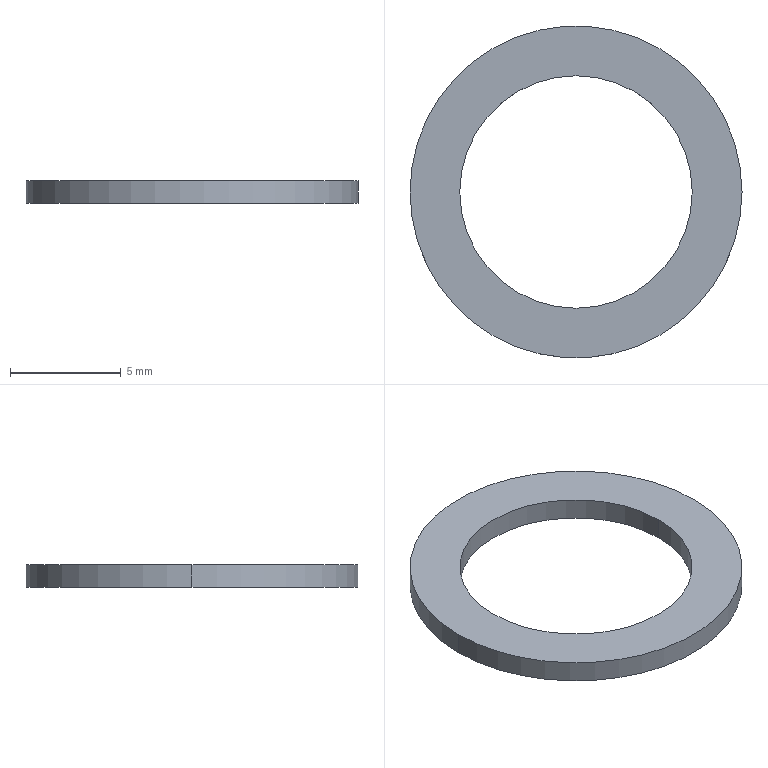Part | STEP file | BCC3 H11_5 | 1 solid | 6 faces | box 15 x 15 x 1 mm | volume 90.124 mm3 | cylinder 4 | plane 2 | commonest cylinder face diameters 10.5 x2 15 x2
STEP:
#1=CARTESIAN_POINT('',(0.,0.,0.));
#2=DIRECTION('',(0.,0.,1.));
#3=DIRECTION('',(1.,0.,0.));
#4=AXIS2_PLACEMENT_3D('',#1,#2,#3);
#5=CARTESIAN_POINT('',(-5.25,0.,1.));
#6=VERTEX_POINT('',#5);
#7=CARTESIAN_POINT('',(-5.25,0.,0.));
#8=VERTEX_POINT('',#7);
#9=CARTESIAN_POINT('',(-5.25,0.,1.));
#10=DIRECTION('',(0.,0.,-1.));
#11=VECTOR('',#10,1.);
#12=LINE('',#9,#11);
#13=CARTESIAN_POINT('',(0.,0.,1.));
#14=DIRECTION('',(0.,0.,-1.));
#15=DIRECTION('',(-1.,0.,0.));
#16=AXIS2_PLACEMENT_3D('',#13,#14,#15);
#17=CYLINDRICAL_SURFACE('',#16,5.25);
#18=CARTESIAN_POINT('',(6.283,0.));
#19=DIRECTION('',(0.,1.));
#20=VECTOR('',#19,1.);
#21=LINE('',#18,#20);
#22=(GEOMETRIC_REPRESENTATION_CONTEXT(2)PARAMETRIC_REPRESENTATION_CONTEXT()REPRESENTATION_CONTEXT('',''));
#23=DEFINITIONAL_REPRESENTATION('',(#21),#22);
#24=PCURVE('',#17,#23);
#25=CARTESIAN_POINT('',(0.,0.,1.));
#26=DIRECTION('',(0.,0.,-1.));
#27=DIRECTION('',(-1.,0.,0.));
#28=AXIS2_PLACEMENT_3D('',#25,#26,#27);
#29=CYLINDRICAL_SURFACE('',#28,5.25);
#30=CARTESIAN_POINT('',(0.,0.));
#31=DIRECTION('',(0.,1.));
#32=VECTOR('',#31,1.);
#33=LINE('',#30,#32);
#34=(GEOMETRIC_REPRESENTATION_CONTEXT(2)PARAMETRIC_REPRESENTATION_CONTEXT()REPRESENTATION_CONTEXT('',''));
#35=DEFINITIONAL_REPRESENTATION('',(#33),#34);
#36=PCURVE('',#29,#35);
#37=SURFACE_CURVE('',#12,(#24,#36),.PCURVE_S1.);
#38=EDGE_CURVE('',#6,#8,#37,.T.);
#39=ORIENTED_EDGE('',*,*,#38,.T.);
#40=CARTESIAN_POINT('',(5.25,0.,0.));
#41=VERTEX_POINT('',#40);
#42=CARTESIAN_POINT('',(0.,0.,0.));
#43=DIRECTION('',(0.,0.,1.));
#44=DIRECTION('',(1.,0.,0.));
#45=AXIS2_PLACEMENT_3D('',#42,#43,#44);
#46=CIRCLE('',#45,5.25);
#47=CARTESIAN_POINT('',(9.425,1.));
#48=DIRECTION('',(-1.,0.));
#49=VECTOR('',#48,1.);
#50=LINE('',#47,#49);
#51=(GEOMETRIC_REPRESENTATION_CONTEXT(2)PARAMETRIC_REPRESENTATION_CONTEXT()REPRESENTATION_CONTEXT('',''));
#52=DEFINITIONAL_REPRESENTATION('',(#50),#51);
#53=PCURVE('',#17,#52);
#54=CARTESIAN_POINT('',(0.,0.,0.));
#55=DIRECTION('',(0.,0.,1.));
#56=DIRECTION('',(1.,0.,0.));
#57=AXIS2_PLACEMENT_3D('',#54,#55,#56);
#58=PLANE('',#57);
#59=CARTESIAN_POINT('',(0.,0.));
#60=DIRECTION('',(1.,0.));
#61=AXIS2_PLACEMENT_2D('',#59,#60);
#62=CIRCLE('',#61,5.25);
#63=(GEOMETRIC_REPRESENTATION_CONTEXT(2)PARAMETRIC_REPRESENTATION_CONTEXT()REPRESENTATION_CONTEXT('',''));
#64=DEFINITIONAL_REPRESENTATION('',(#62),#63);
#65=PCURVE('',#58,#64);
#66=SURFACE_CURVE('',#46,(#53,#65),.PCURVE_S1.);
#67=EDGE_CURVE('',#8,#41,#66,.T.);
#68=ORIENTED_EDGE('',*,*,#67,.T.);
#69=CARTESIAN_POINT('',(5.25,0.,1.));
#70=VERTEX_POINT('',#69);
#71=CARTESIAN_POINT('',(5.25,0.,1.));
#72=DIRECTION('',(0.,0.,-1.));
#73=VECTOR('',#72,1.);
#74=LINE('',#71,#73);
#75=CARTESIAN_POINT('',(3.142,0.));
#76=DIRECTION('',(0.,1.));
#77=VECTOR('',#76,1.);
#78=LINE('',#75,#77);
#79=(GEOMETRIC_REPRESENTATION_CONTEXT(2)PARAMETRIC_REPRESENTATION_CONTEXT()REPRESENTATION_CONTEXT('',''));
#80=DEFINITIONAL_REPRESENTATION('',(#78),#79);
#81=PCURVE('',#17,#80);
#82=CARTESIAN_POINT('',(3.142,0.));
#83=DIRECTION('',(0.,1.));
#84=VECTOR('',#83,1.);
#85=LINE('',#82,#84);
#86=(GEOMETRIC_REPRESENTATION_CONTEXT(2)PARAMETRIC_REPRESENTATION_CONTEXT()REPRESENTATION_CONTEXT('',''));
#87=DEFINITIONAL_REPRESENTATION('',(#85),#86);
#88=PCURVE('',#29,#87);
#89=SURFACE_CURVE('',#74,(#81,#88),.PCURVE_S1.);
#90=EDGE_CURVE('',#70,#41,#89,.T.);
#91=ORIENTED_EDGE('',*,*,#90,.F.);
#92=CARTESIAN_POINT('',(0.,0.,1.));
#93=DIRECTION('',(0.,0.,1.));
#94=DIRECTION('',(1.,0.,0.));
#95=AXIS2_PLACEMENT_3D('',#92,#93,#94);
#96=CIRCLE('',#95,5.25);
#97=CARTESIAN_POINT('',(9.425,0.));
#98=DIRECTION('',(-1.,0.));
#99=VECTOR('',#98,1.);
#100=LINE('',#97,#99);
#101=(GEOMETRIC_REPRESENTATION_CONTEXT(2)PARAMETRIC_REPRESENTATION_CONTEXT()REPRESENTATION_CONTEXT('',''));
#102=DEFINITIONAL_REPRESENTATION('',(#100),#101);
#103=PCURVE('',#17,#102);
#104=CARTESIAN_POINT('',(0.,0.,1.));
#105=DIRECTION('',(0.,0.,1.));
#106=DIRECTION('',(1.,0.,0.));
#107=AXIS2_PLACEMENT_3D('',#104,#105,#106);
#108=PLANE('',#107);
#109=CARTESIAN_POINT('',(0.,0.));
#110=DIRECTION('',(1.,0.));
#111=AXIS2_PLACEMENT_2D('',#109,#110);
#112=CIRCLE('',#111,5.25);
#113=(GEOMETRIC_REPRESENTATION_CONTEXT(2)PARAMETRIC_REPRESENTATION_CONTEXT()REPRESENTATION_CONTEXT('',''));
#114=DEFINITIONAL_REPRESENTATION('',(#112),#113);
#115=PCURVE('',#108,#114);
#116=SURFACE_CURVE('',#96,(#103,#115),.PCURVE_S1.);
#117=EDGE_CURVE('',#6,#70,#116,.T.);
#118=ORIENTED_EDGE('',*,*,#117,.F.);
#119=EDGE_LOOP('',(#39,#68,#91,#118));
#120=FACE_BOUND('',#119,.F.);
#121=ADVANCED_FACE('',(#120),#17,.F.);
#122=CARTESIAN_POINT('',(7.5,0.,1.));
#123=VERTEX_POINT('',#122);
#124=CARTESIAN_POINT('',(-7.5,0.,1.));
#125=VERTEX_POINT('',#124);
#126=CARTESIAN_POINT('',(0.,0.,1.));
#127=DIRECTION('',(0.,0.,1.));
#128=DIRECTION('',(1.,0.,0.));
#129=AXIS2_PLACEMENT_3D('',#126,#127,#128);
#130=CIRCLE('',#129,7.5);
#131=CARTESIAN_POINT('',(0.,0.,1.));
#132=DIRECTION('',(0.,0.,-1.));
#133=DIRECTION('',(-1.,0.,0.));
#134=AXIS2_PLACEMENT_3D('',#131,#132,#133);
#135=CYLINDRICAL_SURFACE('',#134,7.5);
#136=CARTESIAN_POINT('',(3.142,0.));
#137=DIRECTION('',(-1.,0.));
#138=VECTOR('',#137,1.);
#139=LINE('',#136,#138);
#140=(GEOMETRIC_REPRESENTATION_CONTEXT(2)PARAMETRIC_REPRESENTATION_CONTEXT()REPRESENTATION_CONTEXT('',''));
#141=DEFINITIONAL_REPRESENTATION('',(#139),#140);
#142=PCURVE('',#135,#141);
#143=CARTESIAN_POINT('',(0.,0.));
#144=DIRECTION('',(1.,0.));
#145=AXIS2_PLACEMENT_2D('',#143,#144);
#146=CIRCLE('',#145,7.5);
#147=(GEOMETRIC_REPRESENTATION_CONTEXT(2)PARAMETRIC_REPRESENTATION_CONTEXT()REPRESENTATION_CONTEXT('',''));
#148=DEFINITIONAL_REPRESENTATION('',(#146),#147);
#149=PCURVE('',#108,#148);
#150=SURFACE_CURVE('',#130,(#142,#149),.PCURVE_S1.);
#151=EDGE_CURVE('',#123,#125,#150,.T.);
#152=ORIENTED_EDGE('',*,*,#151,.F.);
#153=CARTESIAN_POINT('',(7.5,0.,0.));
#154=VERTEX_POINT('',#153);
#155=CARTESIAN_POINT('',(7.5,0.,1.));
#156=DIRECTION('',(0.,0.,-1.));
#157=VECTOR('',#156,1.);
#158=LINE('',#155,#157);
#159=CARTESIAN_POINT('',(3.142,0.));
#160=DIRECTION('',(0.,1.));
#161=VECTOR('',#160,1.);
#162=LINE('',#159,#161);
#163=(GEOMETRIC_REPRESENTATION_CONTEXT(2)PARAMETRIC_REPRESENTATION_CONTEXT()REPRESENTATION_CONTEXT('',''));
#164=DEFINITIONAL_REPRESENTATION('',(#162),#163);
#165=PCURVE('',#135,#164);
#166=CARTESIAN_POINT('',(0.,0.,1.));
#167=DIRECTION('',(0.,0.,-1.));
#168=DIRECTION('',(-1.,0.,0.));
#169=AXIS2_PLACEMENT_3D('',#166,#167,#168);
#170=CYLINDRICAL_SURFACE('',#169,7.5);
#171=CARTESIAN_POINT('',(3.142,0.));
#172=DIRECTION('',(0.,1.));
#173=VECTOR('',#172,1.);
#174=LINE('',#171,#173);
#175=(GEOMETRIC_REPRESENTATION_CONTEXT(2)PARAMETRIC_REPRESENTATION_CONTEXT()REPRESENTATION_CONTEXT('',''));
#176=DEFINITIONAL_REPRESENTATION('',(#174),#175);
#177=PCURVE('',#170,#176);
#178=SURFACE_CURVE('',#158,(#165,#177),.PCURVE_S1.);
#179=EDGE_CURVE('',#123,#154,#178,.T.);
#180=ORIENTED_EDGE('',*,*,#179,.T.);
#181=CARTESIAN_POINT('',(-7.5,0.,0.));
#182=VERTEX_POINT('',#181);
#183=CARTESIAN_POINT('',(0.,0.,0.));
#184=DIRECTION('',(0.,0.,1.));
#185=DIRECTION('',(1.,0.,0.));
#186=AXIS2_PLACEMENT_3D('',#183,#184,#185);
#187=CIRCLE('',#186,7.5);
#188=CARTESIAN_POINT('',(3.142,1.));
#189=DIRECTION('',(-1.,0.));
#190=VECTOR('',#189,1.);
#191=LINE('',#188,#190);
#192=(GEOMETRIC_REPRESENTATION_CONTEXT(2)PARAMETRIC_REPRESENTATION_CONTEXT()REPRESENTATION_CONTEXT('',''));
#193=DEFINITIONAL_REPRESENTATION('',(#191),#192);
#194=PCURVE('',#135,#193);
#195=CARTESIAN_POINT('',(0.,0.));
#196=DIRECTION('',(1.,0.));
#197=AXIS2_PLACEMENT_2D('',#195,#196);
#198=CIRCLE('',#197,7.5);
#199=(GEOMETRIC_REPRESENTATION_CONTEXT(2)PARAMETRIC_REPRESENTATION_CONTEXT()REPRESENTATION_CONTEXT('',''));
#200=DEFINITIONAL_REPRESENTATION('',(#198),#199);
#201=PCURVE('',#58,#200);
#202=SURFACE_CURVE('',#187,(#194,#201),.PCURVE_S1.);
#203=EDGE_CURVE('',#154,#182,#202,.T.);
#204=ORIENTED_EDGE('',*,*,#203,.T.);
#205=CARTESIAN_POINT('',(-7.5,0.,1.));
#206=DIRECTION('',(0.,0.,-1.));
#207=VECTOR('',#206,1.);
#208=LINE('',#205,#207);
#209=CARTESIAN_POINT('',(0.,0.));
#210=DIRECTION('',(0.,1.));
#211=VECTOR('',#210,1.);
#212=LINE('',#209,#211);
#213=(GEOMETRIC_REPRESENTATION_CONTEXT(2)PARAMETRIC_REPRESENTATION_CONTEXT()REPRESENTATION_CONTEXT('',''));
#214=DEFINITIONAL_REPRESENTATION('',(#212),#213);
#215=PCURVE('',#135,#214);
#216=CARTESIAN_POINT('',(6.283,0.));
#217=DIRECTION('',(0.,1.));
#218=VECTOR('',#217,1.);
#219=LINE('',#216,#218);
#220=(GEOMETRIC_REPRESENTATION_CONTEXT(2)PARAMETRIC_REPRESENTATION_CONTEXT()REPRESENTATION_CONTEXT('',''));
#221=DEFINITIONAL_REPRESENTATION('',(#219),#220);
#222=PCURVE('',#170,#221);
#223=SURFACE_CURVE('',#208,(#215,#222),.PCURVE_S1.);
#224=EDGE_CURVE('',#125,#182,#223,.T.);
#225=ORIENTED_EDGE('',*,*,#224,.F.);
#226=EDGE_LOOP('',(#152,#180,#204,#225));
#227=FACE_BOUND('',#226,.T.);
#228=ADVANCED_FACE('',(#227),#135,.T.);
#229=CARTESIAN_POINT('',(0.,0.,1.));
#230=DIRECTION('',(0.,0.,1.));
#231=DIRECTION('',(1.,0.,0.));
#232=AXIS2_PLACEMENT_3D('',#229,#230,#231);
#233=CIRCLE('',#232,7.5);
#234=CARTESIAN_POINT('',(0.,0.));
#235=DIRECTION('',(1.,0.));
#236=AXIS2_PLACEMENT_2D('',#234,#235);
#237=CIRCLE('',#236,7.5);
#238=(GEOMETRIC_REPRESENTATION_CONTEXT(2)PARAMETRIC_REPRESENTATION_CONTEXT()REPRESENTATION_CONTEXT('',''));
#239=DEFINITIONAL_REPRESENTATION('',(#237),#238);
#240=PCURVE('',#108,#239);
#241=CARTESIAN_POINT('',(9.425,0.));
#242=DIRECTION('',(-1.,0.));
#243=VECTOR('',#242,1.);
#244=LINE('',#241,#243);
#245=(GEOMETRIC_REPRESENTATION_CONTEXT(2)PARAMETRIC_REPRESENTATION_CONTEXT()REPRESENTATION_CONTEXT('',''));
#246=DEFINITIONAL_REPRESENTATION('',(#244),#245);
#247=PCURVE('',#170,#246);
#248=SURFACE_CURVE('',#233,(#240,#247),.PCURVE_S1.);
#249=EDGE_CURVE('',#125,#123,#248,.T.);
#250=ORIENTED_EDGE('',*,*,#249,.T.);
#251=ORIENTED_EDGE('',*,*,#151,.T.);
#252=EDGE_LOOP('',(#250,#251));
#253=FACE_BOUND('',#252,.T.);
#254=ORIENTED_EDGE('',*,*,#117,.F.);
#255=CARTESIAN_POINT('',(0.,0.,1.));
#256=DIRECTION('',(0.,0.,1.));
#257=DIRECTION('',(1.,0.,0.));
#258=AXIS2_PLACEMENT_3D('',#255,#256,#257);
#259=CIRCLE('',#258,5.25);
#260=CARTESIAN_POINT('',(0.,0.));
#261=DIRECTION('',(1.,0.));
#262=AXIS2_PLACEMENT_2D('',#260,#261);
#263=CIRCLE('',#262,5.25);
#264=(GEOMETRIC_REPRESENTATION_CONTEXT(2)PARAMETRIC_REPRESENTATION_CONTEXT()REPRESENTATION_CONTEXT('',''));
#265=DEFINITIONAL_REPRESENTATION('',(#263),#264);
#266=PCURVE('',#108,#265);
#267=CARTESIAN_POINT('',(3.142,0.));
#268=DIRECTION('',(-1.,0.));
#269=VECTOR('',#268,1.);
#270=LINE('',#267,#269);
#271=(GEOMETRIC_REPRESENTATION_CONTEXT(2)PARAMETRIC_REPRESENTATION_CONTEXT()REPRESENTATION_CONTEXT('',''));
#272=DEFINITIONAL_REPRESENTATION('',(#270),#271);
#273=PCURVE('',#29,#272);
#274=SURFACE_CURVE('',#259,(#266,#273),.PCURVE_S1.);
#275=EDGE_CURVE('',#70,#6,#274,.T.);
#276=ORIENTED_EDGE('',*,*,#275,.F.);
#277=EDGE_LOOP('',(#254,#276));
#278=FACE_BOUND('',#277,.T.);
#279=ADVANCED_FACE('',(#253,#278),#108,.T.);
#280=CARTESIAN_POINT('',(0.,0.,0.));
#281=DIRECTION('',(0.,0.,1.));
#282=DIRECTION('',(1.,0.,0.));
#283=AXIS2_PLACEMENT_3D('',#280,#281,#282);
#284=CIRCLE('',#283,7.5);
#285=CARTESIAN_POINT('',(0.,0.));
#286=DIRECTION('',(1.,0.));
#287=AXIS2_PLACEMENT_2D('',#285,#286);
#288=CIRCLE('',#287,7.5);
#289=(GEOMETRIC_REPRESENTATION_CONTEXT(2)PARAMETRIC_REPRESENTATION_CONTEXT()REPRESENTATION_CONTEXT('',''));
#290=DEFINITIONAL_REPRESENTATION('',(#288),#289);
#291=PCURVE('',#58,#290);
#292=CARTESIAN_POINT('',(9.425,1.));
#293=DIRECTION('',(-1.,0.));
#294=VECTOR('',#293,1.);
#295=LINE('',#292,#294);
#296=(GEOMETRIC_REPRESENTATION_CONTEXT(2)PARAMETRIC_REPRESENTATION_CONTEXT()REPRESENTATION_CONTEXT('',''));
#297=DEFINITIONAL_REPRESENTATION('',(#295),#296);
#298=PCURVE('',#170,#297);
#299=SURFACE_CURVE('',#284,(#291,#298),.PCURVE_S1.);
#300=EDGE_CURVE('',#182,#154,#299,.T.);
#301=ORIENTED_EDGE('',*,*,#300,.F.);
#302=ORIENTED_EDGE('',*,*,#203,.F.);
#303=EDGE_LOOP('',(#301,#302));
#304=FACE_BOUND('',#303,.T.);
#305=ORIENTED_EDGE('',*,*,#67,.T.);
#306=CARTESIAN_POINT('',(0.,0.,0.));
#307=DIRECTION('',(0.,0.,1.));
#308=DIRECTION('',(1.,0.,0.));
#309=AXIS2_PLACEMENT_3D('',#306,#307,#308);
#310=CIRCLE('',#309,5.25);
#311=CARTESIAN_POINT('',(0.,0.));
#312=DIRECTION('',(1.,0.));
#313=AXIS2_PLACEMENT_2D('',#311,#312);
#314=CIRCLE('',#313,5.25);
#315=(GEOMETRIC_REPRESENTATION_CONTEXT(2)PARAMETRIC_REPRESENTATION_CONTEXT()REPRESENTATION_CONTEXT('',''));
#316=DEFINITIONAL_REPRESENTATION('',(#314),#315);
#317=PCURVE('',#58,#316);
#318=CARTESIAN_POINT('',(3.142,1.));
#319=DIRECTION('',(-1.,0.));
#320=VECTOR('',#319,1.);
#321=LINE('',#318,#320);
#322=(GEOMETRIC_REPRESENTATION_CONTEXT(2)PARAMETRIC_REPRESENTATION_CONTEXT()REPRESENTATION_CONTEXT('',''));
#323=DEFINITIONAL_REPRESENTATION('',(#321),#322);
#324=PCURVE('',#29,#323);
#325=SURFACE_CURVE('',#310,(#317,#324),.PCURVE_S1.);
#326=EDGE_CURVE('',#41,#8,#325,.T.);
#327=ORIENTED_EDGE('',*,*,#326,.T.);
#328=EDGE_LOOP('',(#305,#327));
#329=FACE_BOUND('',#328,.T.);
#330=ADVANCED_FACE('',(#304,#329),#58,.F.);
#331=ORIENTED_EDGE('',*,*,#179,.F.);
#332=ORIENTED_EDGE('',*,*,#249,.F.);
#333=ORIENTED_EDGE('',*,*,#224,.T.);
#334=ORIENTED_EDGE('',*,*,#300,.T.);
#335=EDGE_LOOP('',(#331,#332,#333,#334));
#336=FACE_BOUND('',#335,.T.);
#337=ADVANCED_FACE('',(#336),#170,.T.);
#338=ORIENTED_EDGE('',*,*,#326,.T.);
#339=ORIENTED_EDGE('',*,*,#38,.F.);
#340=ORIENTED_EDGE('',*,*,#275,.F.);
#341=ORIENTED_EDGE('',*,*,#90,.T.);
#342=EDGE_LOOP('',(#338,#339,#340,#341));
#343=FACE_BOUND('',#342,.F.);
#344=ADVANCED_FACE('',(#343),#29,.F.);
#345=CLOSED_SHELL('',(#121,#228,#279,#330,#337,#344));
#346=MANIFOLD_SOLID_BREP('',#345);
#347=(LENGTH_UNIT()NAMED_UNIT(*)SI_UNIT(.MILLI.,.METRE.));
#348=UNCERTAINTY_MEASURE_WITH_UNIT(LENGTH_MEASURE(0.0000001),#347,'','');
#349=(NAMED_UNIT(*)PLANE_ANGLE_UNIT()SI_UNIT($,.RADIAN.));
#350=(NAMED_UNIT(*)SI_UNIT($,.STERADIAN.)SOLID_ANGLE_UNIT());
#351=(GEOMETRIC_REPRESENTATION_CONTEXT(3)GLOBAL_UNCERTAINTY_ASSIGNED_CONTEXT((#348))GLOBAL_UNIT_ASSIGNED_CONTEXT((#347,#349,#350))REPRESENTATION_CONTEXT('',''));
#352=ADVANCED_BREP_SHAPE_REPRESENTATION('',(#4,#346),#351);